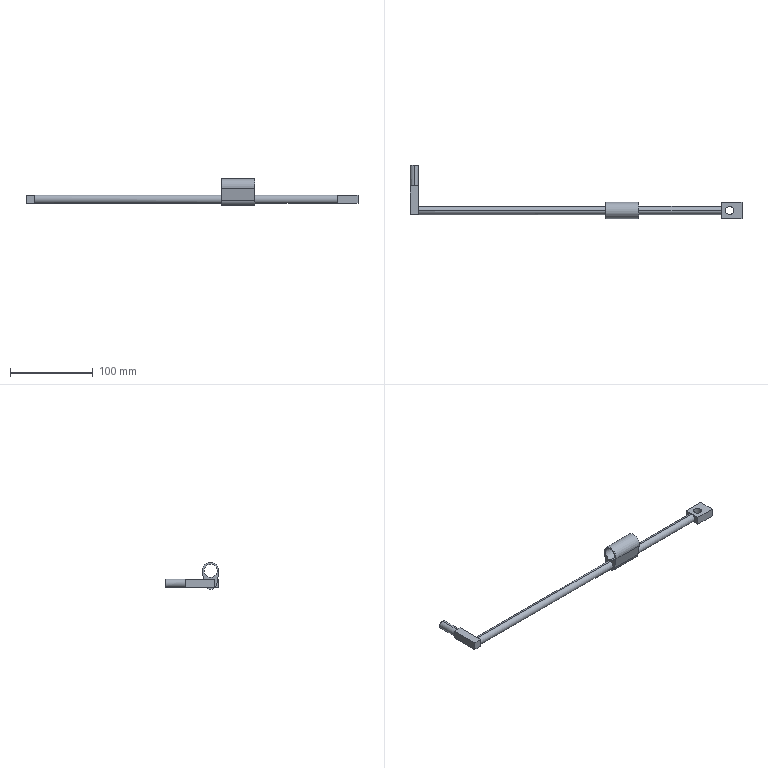Part | SolidWorks | features ICE 4, Extrusion 1, HoleWzd 1 | 1 solid | 40 faces | box 402 x 65 x 32.5 mm | volume 47736 mm3 | plane 23 | cylinder 15 | cone 2 | commonest cylinder face diameters 10 x8 3.3 x2 15 x2 16 x2 20 x1
STEP:
#1=CARTESIAN_POINT('',(-367.,10.,10.));
#2=VERTEX_POINT('',#1);
#3=CARTESIAN_POINT('',(-367.,10.,0.));
#4=VERTEX_POINT('',#3);
#5=CARTESIAN_POINT('',(-367.,10.,5.));
#6=DIRECTION('',(-1.,0.,0.));
#7=DIRECTION('',(0.,0.,1.));
#8=AXIS2_PLACEMENT_3D('',#5,#6,#7);
#9=CIRCLE('',#8,5.);
#10=EDGE_CURVE('',#2,#4,#9,.T.);
#11=ORIENTED_EDGE('',*,*,#10,.F.);
#12=CARTESIAN_POINT('',(-140.,10.,10.));
#13=VERTEX_POINT('',#12);
#14=CARTESIAN_POINT('',(-367.,10.,10.));
#15=DIRECTION('',(1.,0.,0.));
#16=VECTOR('',#15,1000.);
#17=LINE('',#14,#16);
#18=EDGE_CURVE('',#2,#13,#17,.T.);
#19=ORIENTED_EDGE('',*,*,#18,.T.);
#20=CARTESIAN_POINT('',(-140.,10.,0.));
#21=VERTEX_POINT('',#20);
#22=CARTESIAN_POINT('',(-140.,10.,5.));
#23=DIRECTION('',(-1.,0.,0.));
#24=DIRECTION('',(0.,0.,1.));
#25=AXIS2_PLACEMENT_3D('',#22,#23,#24);
#26=CIRCLE('',#25,5.);
#27=EDGE_CURVE('',#13,#21,#26,.T.);
#28=ORIENTED_EDGE('',*,*,#27,.T.);
#29=CARTESIAN_POINT('',(-367.,10.,0.));
#30=DIRECTION('',(1.,0.,0.));
#31=VECTOR('',#30,1000.);
#32=LINE('',#29,#31);
#33=EDGE_CURVE('',#4,#21,#32,.T.);
#34=ORIENTED_EDGE('',*,*,#33,.F.);
#35=EDGE_LOOP('',(#11,#19,#28,#34));
#36=FACE_OUTER_BOUND('',#35,.T.);
#37=CARTESIAN_POINT('',(-367.,10.,5.));
#38=DIRECTION('',(1.,0.,0.));
#39=DIRECTION('',(0.,0.,-1.));
#40=AXIS2_PLACEMENT_3D('',#37,#38,#39);
#41=CYLINDRICAL_SURFACE('',#40,5.);
#42=ADVANCED_FACE('',(#36),#41,.T.);
#43=CARTESIAN_POINT('',(-372.,65.,10.));
#44=VERTEX_POINT('',#43);
#45=CARTESIAN_POINT('',(-372.,65.,0.));
#46=VERTEX_POINT('',#45);
#47=CARTESIAN_POINT('',(-372.,65.,5.));
#48=DIRECTION('',(0.,1.,0.));
#49=DIRECTION('',(0.,0.,1.));
#50=AXIS2_PLACEMENT_3D('',#47,#48,#49);
#51=CIRCLE('',#50,5.);
#52=EDGE_CURVE('',#44,#46,#51,.T.);
#53=ORIENTED_EDGE('',*,*,#52,.F.);
#54=CARTESIAN_POINT('',(-372.,40.,10.));
#55=VERTEX_POINT('',#54);
#56=CARTESIAN_POINT('',(-372.,65.,10.));
#57=DIRECTION('',(0.,-1.,0.));
#58=VECTOR('',#57,1000.);
#59=LINE('',#56,#58);
#60=EDGE_CURVE('',#44,#55,#59,.T.);
#61=ORIENTED_EDGE('',*,*,#60,.T.);
#62=CARTESIAN_POINT('',(-367.,40.,5.));
#63=VERTEX_POINT('',#62);
#64=CARTESIAN_POINT('',(-372.,40.,5.));
#65=DIRECTION('',(0.,1.,0.));
#66=DIRECTION('',(0.,0.,1.));
#67=AXIS2_PLACEMENT_3D('',#64,#65,#66);
#68=CIRCLE('',#67,5.);
#69=EDGE_CURVE('',#55,#63,#68,.T.);
#70=ORIENTED_EDGE('',*,*,#69,.T.);
#71=CARTESIAN_POINT('',(-372.,40.,0.));
#72=VERTEX_POINT('',#71);
#73=CARTESIAN_POINT('',(-372.,40.,5.));
#74=DIRECTION('',(0.,1.,0.));
#75=DIRECTION('',(0.,0.,1.));
#76=AXIS2_PLACEMENT_3D('',#73,#74,#75);
#77=CIRCLE('',#76,5.);
#78=EDGE_CURVE('',#63,#72,#77,.T.);
#79=ORIENTED_EDGE('',*,*,#78,.T.);
#80=CARTESIAN_POINT('',(-372.,65.,0.));
#81=DIRECTION('',(0.,-1.,0.));
#82=VECTOR('',#81,1000.);
#83=LINE('',#80,#82);
#84=EDGE_CURVE('',#46,#72,#83,.T.);
#85=ORIENTED_EDGE('',*,*,#84,.F.);
#86=EDGE_LOOP('',(#53,#61,#70,#79,#85));
#87=FACE_OUTER_BOUND('',#86,.T.);
#88=CARTESIAN_POINT('',(-372.,65.,5.));
#89=DIRECTION('',(0.,-1.,0.));
#90=DIRECTION('',(0.,0.,-1.));
#91=AXIS2_PLACEMENT_3D('',#88,#89,#90);
#92=CYLINDRICAL_SURFACE('',#91,5.);
#93=ADVANCED_FACE('',(#87),#92,.T.);
#94=CARTESIAN_POINT('',(-140.,10.,12.));
#95=VERTEX_POINT('',#94);
#96=CARTESIAN_POINT('',(-140.,10.,28.));
#97=VERTEX_POINT('',#96);
#98=CARTESIAN_POINT('',(-140.,10.,20.));
#99=DIRECTION('',(-1.,0.,0.));
#100=DIRECTION('',(0.,0.,1.));
#101=AXIS2_PLACEMENT_3D('',#98,#99,#100);
#102=CIRCLE('',#101,8.);
#103=EDGE_CURVE('',#95,#97,#102,.T.);
#104=ORIENTED_EDGE('',*,*,#103,.T.);
#105=CARTESIAN_POINT('',(-100.,10.,28.));
#106=VERTEX_POINT('',#105);
#107=CARTESIAN_POINT('',(-140.,10.,28.));
#108=DIRECTION('',(1.,0.,0.));
#109=VECTOR('',#108,1000.);
#110=LINE('',#107,#109);
#111=EDGE_CURVE('',#97,#106,#110,.T.);
#112=ORIENTED_EDGE('',*,*,#111,.T.);
#113=CARTESIAN_POINT('',(-100.,10.,12.));
#114=VERTEX_POINT('',#113);
#115=CARTESIAN_POINT('',(-100.,10.,20.));
#116=DIRECTION('',(-1.,0.,0.));
#117=DIRECTION('',(0.,0.,1.));
#118=AXIS2_PLACEMENT_3D('',#115,#116,#117);
#119=CIRCLE('',#118,8.);
#120=EDGE_CURVE('',#114,#106,#119,.T.);
#121=ORIENTED_EDGE('',*,*,#120,.F.);
#122=CARTESIAN_POINT('',(-140.,10.,12.));
#123=DIRECTION('',(1.,0.,0.));
#124=VECTOR('',#123,1000.);
#125=LINE('',#122,#124);
#126=EDGE_CURVE('',#95,#114,#125,.T.);
#127=ORIENTED_EDGE('',*,*,#126,.F.);
#128=EDGE_LOOP('',(#104,#112,#121,#127));
#129=FACE_OUTER_BOUND('',#128,.T.);
#130=CARTESIAN_POINT('',(-140.,10.,20.));
#131=DIRECTION('',(1.,0.,0.));
#132=DIRECTION('',(0.,0.,-1.));
#133=AXIS2_PLACEMENT_3D('',#130,#131,#132);
#134=CYLINDRICAL_SURFACE('',#133,8.);
#135=ADVANCED_FACE('',(#129),#134,.F.);
#136=CARTESIAN_POINT('',(-140.,10.,-2.5));
#137=VERTEX_POINT('',#136);
#138=CARTESIAN_POINT('',(-140.,2.605,3.75));
#139=VERTEX_POINT('',#138);
#140=CARTESIAN_POINT('',(-140.,10.,5.));
#141=DIRECTION('',(-1.,0.,0.));
#142=DIRECTION('',(0.,0.,1.));
#143=AXIS2_PLACEMENT_3D('',#140,#141,#142);
#144=CIRCLE('',#143,7.5);
#145=EDGE_CURVE('',#137,#139,#144,.T.);
#146=ORIENTED_EDGE('',*,*,#145,.F.);
#147=CARTESIAN_POINT('',(-100.,10.,-2.5));
#148=VERTEX_POINT('',#147);
#149=CARTESIAN_POINT('',(-140.,10.,-2.5));
#150=DIRECTION('',(1.,0.,0.));
#151=VECTOR('',#150,1000.);
#152=LINE('',#149,#151);
#153=EDGE_CURVE('',#137,#148,#152,.T.);
#154=ORIENTED_EDGE('',*,*,#153,.T.);
#155=CARTESIAN_POINT('',(-100.,2.605,3.75));
#156=VERTEX_POINT('',#155);
#157=CARTESIAN_POINT('',(-100.,10.,5.));
#158=DIRECTION('',(-1.,0.,0.));
#159=DIRECTION('',(0.,0.,1.));
#160=AXIS2_PLACEMENT_3D('',#157,#158,#159);
#161=CIRCLE('',#160,7.5);
#162=EDGE_CURVE('',#148,#156,#161,.T.);
#163=ORIENTED_EDGE('',*,*,#162,.T.);
#164=CARTESIAN_POINT('',(-140.,2.605,3.75));
#165=DIRECTION('',(1.,0.,0.));
#166=VECTOR('',#165,1000.);
#167=LINE('',#164,#166);
#168=EDGE_CURVE('',#139,#156,#167,.T.);
#169=ORIENTED_EDGE('',*,*,#168,.F.);
#170=EDGE_LOOP('',(#146,#154,#163,#169));
#171=FACE_OUTER_BOUND('',#170,.T.);
#172=CARTESIAN_POINT('',(-140.,10.,5.));
#173=DIRECTION('',(1.,0.,0.));
#174=DIRECTION('',(0.,0.,-1.));
#175=AXIS2_PLACEMENT_3D('',#172,#173,#174);
#176=CYLINDRICAL_SURFACE('',#175,7.5);
#177=ADVANCED_FACE('',(#171),#176,.T.);
#178=CARTESIAN_POINT('',(20.,10.,6.65));
#179=VERTEX_POINT('',#178);
#180=CARTESIAN_POINT('',(20.,10.,3.35));
#181=VERTEX_POINT('',#180);
#182=CARTESIAN_POINT('',(20.,10.,5.));
#183=DIRECTION('',(1.,0.,0.));
#184=DIRECTION('',(0.,0.,-1.));
#185=AXIS2_PLACEMENT_3D('',#182,#183,#184);
#186=CIRCLE('',#185,1.65);
#187=EDGE_CURVE('',#179,#181,#186,.T.);
#188=ORIENTED_EDGE('',*,*,#187,.F.);
#189=CARTESIAN_POINT('',(25.,10.,6.65));
#190=VERTEX_POINT('',#189);
#191=CARTESIAN_POINT('',(25.,10.,6.65));
#192=DIRECTION('',(1.,0.,0.));
#193=VECTOR('',#192,1000.);
#194=LINE('',#191,#193);
#195=EDGE_CURVE('',#179,#190,#194,.T.);
#196=ORIENTED_EDGE('',*,*,#195,.T.);
#197=CARTESIAN_POINT('',(25.,10.,3.35));
#198=VERTEX_POINT('',#197);
#199=CARTESIAN_POINT('',(25.,10.,5.));
#200=DIRECTION('',(1.,0.,0.));
#201=DIRECTION('',(0.,0.,-1.));
#202=AXIS2_PLACEMENT_3D('',#199,#200,#201);
#203=CIRCLE('',#202,1.65);
#204=EDGE_CURVE('',#190,#198,#203,.T.);
#205=ORIENTED_EDGE('',*,*,#204,.T.);
#206=CARTESIAN_POINT('',(25.,10.,3.35));
#207=DIRECTION('',(1.,0.,0.));
#208=VECTOR('',#207,1000.);
#209=LINE('',#206,#208);
#210=EDGE_CURVE('',#181,#198,#209,.T.);
#211=ORIENTED_EDGE('',*,*,#210,.F.);
#212=EDGE_LOOP('',(#188,#196,#205,#211));
#213=FACE_OUTER_BOUND('',#212,.T.);
#214=CARTESIAN_POINT('',(25.,10.,5.));
#215=DIRECTION('',(1.,0.,0.));
#216=DIRECTION('',(0.,0.,-1.));
#217=AXIS2_PLACEMENT_3D('',#214,#215,#216);
#218=CYLINDRICAL_SURFACE('',#217,1.65);
#219=ADVANCED_FACE('',(#213),#218,.F.);
#220=CARTESIAN_POINT('',(19.009,10.,5.));
#221=VERTEX_POINT('',#220);
#222=CARTESIAN_POINT('',(20.,10.,3.35));
#223=DIRECTION('',(0.515,0.,-0.8572));
#224=VECTOR('',#223,1000.);
#225=LINE('',#222,#224);
#226=EDGE_CURVE('',#221,#181,#225,.T.);
#227=ORIENTED_EDGE('',*,*,#226,.F.);
#228=CARTESIAN_POINT('',(20.,10.,6.65));
#229=DIRECTION('',(0.515,0.,0.8572));
#230=VECTOR('',#229,1000.);
#231=LINE('',#228,#230);
#232=EDGE_CURVE('',#221,#179,#231,.T.);
#233=ORIENTED_EDGE('',*,*,#232,.T.);
#234=ORIENTED_EDGE('',*,*,#187,.T.);
#235=EDGE_LOOP('',(#227,#233,#234));
#236=FACE_OUTER_BOUND('',#235,.T.);
#237=CARTESIAN_POINT('',(20.,10.,5.));
#238=DIRECTION('',(1.,0.,0.));
#239=DIRECTION('',(0.,0.,-1.));
#240=AXIS2_PLACEMENT_3D('',#237,#238,#239);
#241=CONICAL_SURFACE('',#240,1.65,1.03);
#242=ADVANCED_FACE('',(#236),#241,.F.);
#243=CARTESIAN_POINT('',(5.,10.,10.));
#244=VERTEX_POINT('',#243);
#245=CARTESIAN_POINT('',(15.,10.,10.));
#246=VERTEX_POINT('',#245);
#247=CARTESIAN_POINT('',(10.,10.,10.));
#248=DIRECTION('',(0.,0.,1.));
#249=DIRECTION('',(1.,0.,0.));
#250=AXIS2_PLACEMENT_3D('',#247,#248,#249);
#251=CIRCLE('',#250,5.);
#252=EDGE_CURVE('',#244,#246,#251,.T.);
#253=ORIENTED_EDGE('',*,*,#252,.T.);
#254=CARTESIAN_POINT('',(15.,10.,0.));
#255=VERTEX_POINT('',#254);
#256=CARTESIAN_POINT('',(15.,10.,10.));
#257=DIRECTION('',(0.,0.,-1.));
#258=VECTOR('',#257,1000.);
#259=LINE('',#256,#258);
#260=EDGE_CURVE('',#246,#255,#259,.T.);
#261=ORIENTED_EDGE('',*,*,#260,.T.);
#262=CARTESIAN_POINT('',(5.,10.,0.));
#263=VERTEX_POINT('',#262);
#264=CARTESIAN_POINT('',(10.,10.,0.));
#265=DIRECTION('',(0.,0.,1.));
#266=DIRECTION('',(1.,0.,0.));
#267=AXIS2_PLACEMENT_3D('',#264,#265,#266);
#268=CIRCLE('',#267,5.);
#269=EDGE_CURVE('',#263,#255,#268,.T.);
#270=ORIENTED_EDGE('',*,*,#269,.F.);
#271=CARTESIAN_POINT('',(5.,10.,10.));
#272=DIRECTION('',(0.,0.,-1.));
#273=VECTOR('',#272,1000.);
#274=LINE('',#271,#273);
#275=EDGE_CURVE('',#244,#263,#274,.T.);
#276=ORIENTED_EDGE('',*,*,#275,.F.);
#277=EDGE_LOOP('',(#253,#261,#270,#276));
#278=FACE_OUTER_BOUND('',#277,.T.);
#279=CARTESIAN_POINT('',(10.,10.,10.));
#280=DIRECTION('',(0.,0.,-1.));
#281=DIRECTION('',(-1.,0.,0.));
#282=AXIS2_PLACEMENT_3D('',#279,#280,#281);
#283=CYLINDRICAL_SURFACE('',#282,5.);
#284=ADVANCED_FACE('',(#278),#283,.F.);
#285=CARTESIAN_POINT('',(-100.,10.,10.));
#286=VERTEX_POINT('',#285);
#287=CARTESIAN_POINT('',(-100.,10.,0.));
#288=VERTEX_POINT('',#287);
#289=CARTESIAN_POINT('',(-100.,10.,5.));
#290=DIRECTION('',(-1.,0.,0.));
#291=DIRECTION('',(0.,0.,1.));
#292=AXIS2_PLACEMENT_3D('',#289,#290,#291);
#293=CIRCLE('',#292,5.);
#294=EDGE_CURVE('',#286,#288,#293,.T.);
#295=ORIENTED_EDGE('',*,*,#294,.F.);
#296=CARTESIAN_POINT('',(0.,10.,10.));
#297=VERTEX_POINT('',#296);
#298=CARTESIAN_POINT('',(-367.,10.,10.));
#299=DIRECTION('',(1.,0.,0.));
#300=VECTOR('',#299,1000.);
#301=LINE('',#298,#300);
#302=EDGE_CURVE('',#286,#297,#301,.T.);
#303=ORIENTED_EDGE('',*,*,#302,.T.);
#304=CARTESIAN_POINT('',(0.,10.,0.));
#305=VERTEX_POINT('',#304);
#306=CARTESIAN_POINT('',(0.,10.,5.));
#307=DIRECTION('',(-1.,0.,0.));
#308=DIRECTION('',(0.,0.,1.));
#309=AXIS2_PLACEMENT_3D('',#306,#307,#308);
#310=CIRCLE('',#309,5.);
#311=EDGE_CURVE('',#297,#305,#310,.T.);
#312=ORIENTED_EDGE('',*,*,#311,.T.);
#313=CARTESIAN_POINT('',(-367.,10.,0.));
#314=DIRECTION('',(1.,0.,0.));
#315=VECTOR('',#314,1000.);
#316=LINE('',#313,#315);
#317=EDGE_CURVE('',#288,#305,#316,.T.);
#318=ORIENTED_EDGE('',*,*,#317,.F.);
#319=EDGE_LOOP('',(#295,#303,#312,#318));
#320=FACE_OUTER_BOUND('',#319,.T.);
#321=CARTESIAN_POINT('',(-367.,10.,5.));
#322=DIRECTION('',(1.,0.,0.));
#323=DIRECTION('',(0.,0.,-1.));
#324=AXIS2_PLACEMENT_3D('',#321,#322,#323);
#325=CYLINDRICAL_SURFACE('',#324,5.);
#326=ADVANCED_FACE('',(#320),#325,.T.);
#327=ORIENTED_EDGE('',*,*,#302,.F.);
#328=CARTESIAN_POINT('',(-100.,10.,5.));
#329=DIRECTION('',(-1.,0.,0.));
#330=DIRECTION('',(0.,0.,1.));
#331=AXIS2_PLACEMENT_3D('',#328,#329,#330);
#332=CIRCLE('',#331,5.);
#333=EDGE_CURVE('',#288,#286,#332,.T.);
#334=ORIENTED_EDGE('',*,*,#333,.F.);
#335=ORIENTED_EDGE('',*,*,#317,.T.);
#336=CARTESIAN_POINT('',(0.,10.,5.));
#337=DIRECTION('',(-1.,0.,0.));
#338=DIRECTION('',(0.,0.,1.));
#339=AXIS2_PLACEMENT_3D('',#336,#337,#338);
#340=CIRCLE('',#339,5.);
#341=EDGE_CURVE('',#305,#297,#340,.T.);
#342=ORIENTED_EDGE('',*,*,#341,.T.);
#343=EDGE_LOOP('',(#327,#334,#335,#342));
#344=FACE_OUTER_BOUND('',#343,.T.);
#345=CARTESIAN_POINT('',(-367.,10.,5.));
#346=DIRECTION('',(1.,0.,0.));
#347=DIRECTION('',(0.,0.,-1.));
#348=AXIS2_PLACEMENT_3D('',#345,#346,#347);
#349=CYLINDRICAL_SURFACE('',#348,5.);
#350=ADVANCED_FACE('',(#344),#349,.T.);
#351=ORIENTED_EDGE('',*,*,#311,.F.);
#352=CARTESIAN_POINT('',(0.,20.,10.));
#353=VERTEX_POINT('',#352);
#354=CARTESIAN_POINT('',(0.,0.,10.));
#355=DIRECTION('',(0.,-1.,0.));
#356=VECTOR('',#355,1000.);
#357=LINE('',#354,#356);
#358=EDGE_CURVE('',#353,#297,#357,.T.);
#359=ORIENTED_EDGE('',*,*,#358,.F.);
#360=CARTESIAN_POINT('',(0.,20.,0.));
#361=VERTEX_POINT('',#360);
#362=CARTESIAN_POINT('',(0.,20.,10.));
#363=DIRECTION('',(0.,0.,-1.));
#364=VECTOR('',#363,1000.);
#365=LINE('',#362,#364);
#366=EDGE_CURVE('',#353,#361,#365,.T.);
#367=ORIENTED_EDGE('',*,*,#366,.T.);
#368=CARTESIAN_POINT('',(0.,0.,0.));
#369=DIRECTION('',(0.,-1.,0.));
#370=VECTOR('',#369,1000.);
#371=LINE('',#368,#370);
#372=EDGE_CURVE('',#361,#305,#371,.T.);
#373=ORIENTED_EDGE('',*,*,#372,.T.);
#374=EDGE_LOOP('',(#351,#359,#367,#373));
#375=FACE_OUTER_BOUND('',#374,.T.);
#376=CARTESIAN_POINT('',(0.,0.,10.));
#377=DIRECTION('',(1.,0.,0.));
#378=DIRECTION('',(0.,0.,-1.));
#379=AXIS2_PLACEMENT_3D('',#376,#377,#378);
#380=PLANE('',#379);
#381=ADVANCED_FACE('',(#375),#380,.F.);
#382=ORIENTED_EDGE('',*,*,#341,.F.);
#383=CARTESIAN_POINT('',(0.,0.,0.));
#384=VERTEX_POINT('',#383);
#385=CARTESIAN_POINT('',(0.,0.,0.));
#386=DIRECTION('',(0.,-1.,0.));
#387=VECTOR('',#386,1000.);
#388=LINE('',#385,#387);
#389=EDGE_CURVE('',#305,#384,#388,.T.);
#390=ORIENTED_EDGE('',*,*,#389,.T.);
#391=CARTESIAN_POINT('',(0.,0.,10.));
#392=VERTEX_POINT('',#391);
#393=CARTESIAN_POINT('',(0.,0.,10.));
#394=DIRECTION('',(0.,0.,-1.));
#395=VECTOR('',#394,1000.);
#396=LINE('',#393,#395);
#397=EDGE_CURVE('',#392,#384,#396,.T.);
#398=ORIENTED_EDGE('',*,*,#397,.F.);
#399=CARTESIAN_POINT('',(0.,0.,10.));
#400=DIRECTION('',(0.,-1.,0.));
#401=VECTOR('',#400,1000.);
#402=LINE('',#399,#401);
#403=EDGE_CURVE('',#297,#392,#402,.T.);
#404=ORIENTED_EDGE('',*,*,#403,.F.);
#405=EDGE_LOOP('',(#382,#390,#398,#404));
#406=FACE_OUTER_BOUND('',#405,.T.);
#407=CARTESIAN_POINT('',(0.,0.,10.));
#408=DIRECTION('',(1.,0.,0.));
#409=DIRECTION('',(0.,0.,-1.));
#410=AXIS2_PLACEMENT_3D('',#407,#408,#409);
#411=PLANE('',#410);
#412=ADVANCED_FACE('',(#406),#411,.F.);
#413=ORIENTED_EDGE('',*,*,#358,.T.);
#414=ORIENTED_EDGE('',*,*,#403,.T.);
#415=CARTESIAN_POINT('',(25.,0.,10.));
#416=VERTEX_POINT('',#415);
#417=CARTESIAN_POINT('',(0.,0.,10.));
#418=DIRECTION('',(1.,0.,0.));
#419=VECTOR('',#418,1000.);
#420=LINE('',#417,#419);
#421=EDGE_CURVE('',#392,#416,#420,.T.);
#422=ORIENTED_EDGE('',*,*,#421,.T.);
#423=CARTESIAN_POINT('',(25.,20.,10.));
#424=VERTEX_POINT('',#423);
#425=CARTESIAN_POINT('',(25.,0.,10.));
#426=DIRECTION('',(0.,1.,0.));
#427=VECTOR('',#426,1000.);
#428=LINE('',#425,#427);
#429=EDGE_CURVE('',#416,#424,#428,.T.);
#430=ORIENTED_EDGE('',*,*,#429,.T.);
#431=CARTESIAN_POINT('',(0.,20.,10.));
#432=DIRECTION('',(-1.,0.,0.));
#433=VECTOR('',#432,1000.);
#434=LINE('',#431,#433);
#435=EDGE_CURVE('',#424,#353,#434,.T.);
#436=ORIENTED_EDGE('',*,*,#435,.T.);
#437=EDGE_LOOP('',(#413,#414,#422,#430,#436));
#438=FACE_OUTER_BOUND('',#437,.T.);
#439=ORIENTED_EDGE('',*,*,#252,.F.);
#440=CARTESIAN_POINT('',(10.,10.,10.));
#441=DIRECTION('',(0.,0.,1.));
#442=DIRECTION('',(1.,0.,0.));
#443=AXIS2_PLACEMENT_3D('',#440,#441,#442);
#444=CIRCLE('',#443,5.);
#445=EDGE_CURVE('',#246,#244,#444,.T.);
#446=ORIENTED_EDGE('',*,*,#445,.F.);
#447=EDGE_LOOP('',(#439,#446));
#448=FACE_BOUND('',#447,.T.);
#449=CARTESIAN_POINT('',(0.,0.,10.));
#450=DIRECTION('',(0.,0.,-1.));
#451=DIRECTION('',(-1.,0.,0.));
#452=AXIS2_PLACEMENT_3D('',#449,#450,#451);
#453=PLANE('',#452);
#454=ADVANCED_FACE('',(#438,#448),#453,.F.);
#455=ORIENTED_EDGE('',*,*,#372,.F.);
#456=CARTESIAN_POINT('',(25.,20.,0.));
#457=VERTEX_POINT('',#456);
#458=CARTESIAN_POINT('',(0.,20.,0.));
#459=DIRECTION('',(-1.,0.,0.));
#460=VECTOR('',#459,1000.);
#461=LINE('',#458,#460);
#462=EDGE_CURVE('',#457,#361,#461,.T.);
#463=ORIENTED_EDGE('',*,*,#462,.F.);
#464=CARTESIAN_POINT('',(25.,0.,0.));
#465=VERTEX_POINT('',#464);
#466=CARTESIAN_POINT('',(25.,0.,0.));
#467=DIRECTION('',(0.,1.,0.));
#468=VECTOR('',#467,1000.);
#469=LINE('',#466,#468);
#470=EDGE_CURVE('',#465,#457,#469,.T.);
#471=ORIENTED_EDGE('',*,*,#470,.F.);
#472=CARTESIAN_POINT('',(0.,0.,0.));
#473=DIRECTION('',(1.,0.,0.));
#474=VECTOR('',#473,1000.);
#475=LINE('',#472,#474);
#476=EDGE_CURVE('',#384,#465,#475,.T.);
#477=ORIENTED_EDGE('',*,*,#476,.F.);
#478=ORIENTED_EDGE('',*,*,#389,.F.);
#479=EDGE_LOOP('',(#455,#463,#471,#477,#478));
#480=FACE_OUTER_BOUND('',#479,.T.);
#481=ORIENTED_EDGE('',*,*,#269,.T.);
#482=CARTESIAN_POINT('',(10.,10.,0.));
#483=DIRECTION('',(0.,0.,1.));
#484=DIRECTION('',(1.,0.,0.));
#485=AXIS2_PLACEMENT_3D('',#482,#483,#484);
#486=CIRCLE('',#485,5.);
#487=EDGE_CURVE('',#255,#263,#486,.T.);
#488=ORIENTED_EDGE('',*,*,#487,.T.);
#489=EDGE_LOOP('',(#481,#488));
#490=FACE_BOUND('',#489,.T.);
#491=CARTESIAN_POINT('',(0.,0.,0.));
#492=DIRECTION('',(0.,0.,-1.));
#493=DIRECTION('',(-1.,0.,0.));
#494=AXIS2_PLACEMENT_3D('',#491,#492,#493);
#495=PLANE('',#494);
#496=ADVANCED_FACE('',(#480,#490),#495,.T.);
#497=ORIENTED_EDGE('',*,*,#476,.T.);
#498=CARTESIAN_POINT('',(25.,0.,10.));
#499=DIRECTION('',(0.,0.,-1.));
#500=VECTOR('',#499,1000.);
#501=LINE('',#498,#500);
#502=EDGE_CURVE('',#416,#465,#501,.T.);
#503=ORIENTED_EDGE('',*,*,#502,.F.);
#504=ORIENTED_EDGE('',*,*,#421,.F.);
#505=ORIENTED_EDGE('',*,*,#397,.T.);
#506=EDGE_LOOP('',(#497,#503,#504,#505));
#507=FACE_OUTER_BOUND('',#506,.T.);
#508=CARTESIAN_POINT('',(0.,0.,10.));
#509=DIRECTION('',(0.,1.,0.));
#510=DIRECTION('',(0.,0.,1.));
#511=AXIS2_PLACEMENT_3D('',#508,#509,#510);
#512=PLANE('',#511);
#513=ADVANCED_FACE('',(#507),#512,.F.);
#514=CARTESIAN_POINT('',(25.,10.,5.));
#515=DIRECTION('',(1.,0.,0.));
#516=DIRECTION('',(0.,0.,-1.));
#517=AXIS2_PLACEMENT_3D('',#514,#515,#516);
#518=CIRCLE('',#517,1.65);
#519=EDGE_CURVE('',#198,#190,#518,.T.);
#520=ORIENTED_EDGE('',*,*,#519,.F.);
#521=ORIENTED_EDGE('',*,*,#204,.F.);
#522=EDGE_LOOP('',(#520,#521));
#523=FACE_BOUND('',#522,.T.);
#524=ORIENTED_EDGE('',*,*,#470,.T.);
#525=CARTESIAN_POINT('',(25.,20.,10.));
#526=DIRECTION('',(0.,0.,-1.));
#527=VECTOR('',#526,1000.);
#528=LINE('',#525,#527);
#529=EDGE_CURVE('',#424,#457,#528,.T.);
#530=ORIENTED_EDGE('',*,*,#529,.F.);
#531=ORIENTED_EDGE('',*,*,#429,.F.);
#532=ORIENTED_EDGE('',*,*,#502,.T.);
#533=EDGE_LOOP('',(#524,#530,#531,#532));
#534=FACE_OUTER_BOUND('',#533,.T.);
#535=CARTESIAN_POINT('',(25.,0.,10.));
#536=DIRECTION('',(-1.,0.,0.));
#537=DIRECTION('',(0.,0.,1.));
#538=AXIS2_PLACEMENT_3D('',#535,#536,#537);
#539=PLANE('',#538);
#540=ADVANCED_FACE('',(#523,#534),#539,.F.);
#541=ORIENTED_EDGE('',*,*,#462,.T.);
#542=ORIENTED_EDGE('',*,*,#366,.F.);
#543=ORIENTED_EDGE('',*,*,#435,.F.);
#544=ORIENTED_EDGE('',*,*,#529,.T.);
#545=EDGE_LOOP('',(#541,#542,#543,#544));
#546=FACE_OUTER_BOUND('',#545,.T.);
#547=CARTESIAN_POINT('',(0.,20.,10.));
#548=DIRECTION('',(0.,-1.,0.));
#549=DIRECTION('',(0.,0.,-1.));
#550=AXIS2_PLACEMENT_3D('',#547,#548,#549);
#551=PLANE('',#550);
#552=ADVANCED_FACE('',(#546),#551,.F.);
#553=ORIENTED_EDGE('',*,*,#260,.F.);
#554=ORIENTED_EDGE('',*,*,#445,.T.);
#555=ORIENTED_EDGE('',*,*,#275,.T.);
#556=ORIENTED_EDGE('',*,*,#487,.F.);
#557=EDGE_LOOP('',(#553,#554,#555,#556));
#558=FACE_OUTER_BOUND('',#557,.T.);
#559=CARTESIAN_POINT('',(10.,10.,10.));
#560=DIRECTION('',(0.,0.,-1.));
#561=DIRECTION('',(-1.,0.,0.));
#562=AXIS2_PLACEMENT_3D('',#559,#560,#561);
#563=CYLINDRICAL_SURFACE('',#562,5.);
#564=ADVANCED_FACE('',(#558),#563,.F.);
#565=ORIENTED_EDGE('',*,*,#232,.F.);
#566=ORIENTED_EDGE('',*,*,#226,.T.);
#567=CARTESIAN_POINT('',(20.,10.,5.));
#568=DIRECTION('',(1.,0.,0.));
#569=DIRECTION('',(0.,0.,-1.));
#570=AXIS2_PLACEMENT_3D('',#567,#568,#569);
#571=CIRCLE('',#570,1.65);
#572=EDGE_CURVE('',#181,#179,#571,.T.);
#573=ORIENTED_EDGE('',*,*,#572,.T.);
#574=EDGE_LOOP('',(#565,#566,#573));
#575=FACE_OUTER_BOUND('',#574,.T.);
#576=CARTESIAN_POINT('',(20.,10.,5.));
#577=DIRECTION('',(1.,0.,0.));
#578=DIRECTION('',(0.,0.,-1.));
#579=AXIS2_PLACEMENT_3D('',#576,#577,#578);
#580=CONICAL_SURFACE('',#579,1.65,1.03);
#581=ADVANCED_FACE('',(#575),#580,.F.);
#582=ORIENTED_EDGE('',*,*,#195,.F.);
#583=ORIENTED_EDGE('',*,*,#572,.F.);
#584=ORIENTED_EDGE('',*,*,#210,.T.);
#585=ORIENTED_EDGE('',*,*,#519,.T.);
#586=EDGE_LOOP('',(#582,#583,#584,#585));
#587=FACE_OUTER_BOUND('',#586,.T.);
#588=CARTESIAN_POINT('',(25.,10.,5.));
#589=DIRECTION('',(1.,0.,0.));
#590=DIRECTION('',(0.,0.,-1.));
#591=AXIS2_PLACEMENT_3D('',#588,#589,#590);
#592=CYLINDRICAL_SURFACE('',#591,1.65);
#593=ADVANCED_FACE('',(#587),#592,.F.);
#594=ORIENTED_EDGE('',*,*,#103,.F.);
#595=CARTESIAN_POINT('',(-140.,10.,20.));
#596=DIRECTION('',(-1.,0.,0.));
#597=DIRECTION('',(0.,0.,1.));
#598=AXIS2_PLACEMENT_3D('',#595,#596,#597);
#599=CIRCLE('',#598,8.);
#600=EDGE_CURVE('',#97,#95,#599,.T.);
#601=ORIENTED_EDGE('',*,*,#600,.F.);
#602=EDGE_LOOP('',(#594,#601));
#603=FACE_BOUND('',#602,.T.);
#604=CARTESIAN_POINT('',(-140.,17.395,3.75));
#605=VERTEX_POINT('',#604);
#606=CARTESIAN_POINT('',(-140.,10.,5.));
#607=DIRECTION('',(-1.,0.,0.));
#608=DIRECTION('',(0.,0.,1.));
#609=AXIS2_PLACEMENT_3D('',#606,#607,#608);
#610=CIRCLE('',#609,7.5);
#611=EDGE_CURVE('',#605,#137,#610,.T.);
#612=ORIENTED_EDGE('',*,*,#611,.T.);
#613=ORIENTED_EDGE('',*,*,#145,.T.);
#614=CARTESIAN_POINT('',(-140.,0.1399,18.333));
#615=VERTEX_POINT('',#614);
#616=CARTESIAN_POINT('',(-140.,2.605,3.75));
#617=DIRECTION('',(0.,-0.1667,0.986));
#618=VECTOR('',#617,1000.);
#619=LINE('',#616,#618);
#620=EDGE_CURVE('',#139,#615,#619,.T.);
#621=ORIENTED_EDGE('',*,*,#620,.T.);
#622=CARTESIAN_POINT('',(-140.,19.86,18.333));
#623=VERTEX_POINT('',#622);
#624=CARTESIAN_POINT('',(-140.,10.,20.));
#625=DIRECTION('',(-1.,0.,0.));
#626=DIRECTION('',(0.,0.,1.));
#627=AXIS2_PLACEMENT_3D('',#624,#625,#626);
#628=CIRCLE('',#627,10.);
#629=EDGE_CURVE('',#615,#623,#628,.T.);
#630=ORIENTED_EDGE('',*,*,#629,.T.);
#631=CARTESIAN_POINT('',(-140.,17.395,3.75));
#632=DIRECTION('',(0.,-0.1667,-0.986));
#633=VECTOR('',#632,1000.);
#634=LINE('',#631,#633);
#635=EDGE_CURVE('',#623,#605,#634,.T.);
#636=ORIENTED_EDGE('',*,*,#635,.T.);
#637=EDGE_LOOP('',(#612,#613,#621,#630,#636));
#638=FACE_OUTER_BOUND('',#637,.T.);
#639=CARTESIAN_POINT('',(-140.,10.,5.));
#640=DIRECTION('',(-1.,0.,0.));
#641=DIRECTION('',(0.,0.,1.));
#642=AXIS2_PLACEMENT_3D('',#639,#640,#641);
#643=CIRCLE('',#642,5.);
#644=EDGE_CURVE('',#21,#13,#643,.T.);
#645=ORIENTED_EDGE('',*,*,#644,.F.);
#646=ORIENTED_EDGE('',*,*,#27,.F.);
#647=EDGE_LOOP('',(#645,#646));
#648=FACE_BOUND('',#647,.T.);
#649=CARTESIAN_POINT('',(-140.,10.,5.));
#650=DIRECTION('',(-1.,0.,0.));
#651=DIRECTION('',(0.,0.,1.));
#652=AXIS2_PLACEMENT_3D('',#649,#650,#651);
#653=PLANE('',#652);
#654=ADVANCED_FACE('',(#603,#638,#648),#653,.T.);
#655=ORIENTED_EDGE('',*,*,#120,.T.);
#656=CARTESIAN_POINT('',(-100.,10.,20.));
#657=DIRECTION('',(-1.,0.,0.));
#658=DIRECTION('',(0.,0.,1.));
#659=AXIS2_PLACEMENT_3D('',#656,#657,#658);
#660=CIRCLE('',#659,8.);
#661=EDGE_CURVE('',#106,#114,#660,.T.);
#662=ORIENTED_EDGE('',*,*,#661,.T.);
#663=EDGE_LOOP('',(#655,#662));
#664=FACE_BOUND('',#663,.T.);
#665=CARTESIAN_POINT('',(-100.,17.395,3.75));
#666=VERTEX_POINT('',#665);
#667=CARTESIAN_POINT('',(-100.,10.,5.));
#668=DIRECTION('',(-1.,0.,0.));
#669=DIRECTION('',(0.,0.,1.));
#670=AXIS2_PLACEMENT_3D('',#667,#668,#669);
#671=CIRCLE('',#670,7.5);
#672=EDGE_CURVE('',#666,#148,#671,.T.);
#673=ORIENTED_EDGE('',*,*,#672,.F.);
#674=CARTESIAN_POINT('',(-100.,19.86,18.333));
#675=VERTEX_POINT('',#674);
#676=CARTESIAN_POINT('',(-100.,17.395,3.75));
#677=DIRECTION('',(0.,-0.1667,-0.986));
#678=VECTOR('',#677,1000.);
#679=LINE('',#676,#678);
#680=EDGE_CURVE('',#675,#666,#679,.T.);
#681=ORIENTED_EDGE('',*,*,#680,.F.);
#682=CARTESIAN_POINT('',(-100.,0.1399,18.333));
#683=VERTEX_POINT('',#682);
#684=CARTESIAN_POINT('',(-100.,10.,20.));
#685=DIRECTION('',(-1.,0.,0.));
#686=DIRECTION('',(0.,0.,1.));
#687=AXIS2_PLACEMENT_3D('',#684,#685,#686);
#688=CIRCLE('',#687,10.);
#689=EDGE_CURVE('',#683,#675,#688,.T.);
#690=ORIENTED_EDGE('',*,*,#689,.F.);
#691=CARTESIAN_POINT('',(-100.,2.605,3.75));
#692=DIRECTION('',(0.,-0.1667,0.986));
#693=VECTOR('',#692,1000.);
#694=LINE('',#691,#693);
#695=EDGE_CURVE('',#156,#683,#694,.T.);
#696=ORIENTED_EDGE('',*,*,#695,.F.);
#697=ORIENTED_EDGE('',*,*,#162,.F.);
#698=EDGE_LOOP('',(#673,#681,#690,#696,#697));
#699=FACE_OUTER_BOUND('',#698,.T.);
#700=ORIENTED_EDGE('',*,*,#333,.T.);
#701=ORIENTED_EDGE('',*,*,#294,.T.);
#702=EDGE_LOOP('',(#700,#701));
#703=FACE_BOUND('',#702,.T.);
#704=CARTESIAN_POINT('',(-100.,10.,5.));
#705=DIRECTION('',(-1.,0.,0.));
#706=DIRECTION('',(0.,0.,1.));
#707=AXIS2_PLACEMENT_3D('',#704,#705,#706);
#708=PLANE('',#707);
#709=ADVANCED_FACE('',(#664,#699,#703),#708,.F.);
#710=ORIENTED_EDGE('',*,*,#153,.F.);
#711=ORIENTED_EDGE('',*,*,#611,.F.);
#712=CARTESIAN_POINT('',(-140.,17.395,3.75));
#713=DIRECTION('',(1.,0.,0.));
#714=VECTOR('',#713,1000.);
#715=LINE('',#712,#714);
#716=EDGE_CURVE('',#605,#666,#715,.T.);
#717=ORIENTED_EDGE('',*,*,#716,.T.);
#718=ORIENTED_EDGE('',*,*,#672,.T.);
#719=EDGE_LOOP('',(#710,#711,#717,#718));
#720=FACE_OUTER_BOUND('',#719,.T.);
#721=CARTESIAN_POINT('',(-140.,10.,5.));
#722=DIRECTION('',(1.,0.,0.));
#723=DIRECTION('',(0.,0.,-1.));
#724=AXIS2_PLACEMENT_3D('',#721,#722,#723);
#725=CYLINDRICAL_SURFACE('',#724,7.5);
#726=ADVANCED_FACE('',(#720),#725,.T.);
#727=ORIENTED_EDGE('',*,*,#695,.T.);
#728=CARTESIAN_POINT('',(-140.,0.1399,18.333));
#729=DIRECTION('',(1.,0.,0.));
#730=VECTOR('',#729,1000.);
#731=LINE('',#728,#730);
#732=EDGE_CURVE('',#615,#683,#731,.T.);
#733=ORIENTED_EDGE('',*,*,#732,.F.);
#734=ORIENTED_EDGE('',*,*,#620,.F.);
#735=ORIENTED_EDGE('',*,*,#168,.T.);
#736=EDGE_LOOP('',(#727,#733,#734,#735));
#737=FACE_OUTER_BOUND('',#736,.T.);
#738=CARTESIAN_POINT('',(-140.,2.605,3.75));
#739=DIRECTION('',(0.,0.986,0.1667));
#740=DIRECTION('',(0.,-0.1667,0.986));
#741=AXIS2_PLACEMENT_3D('',#738,#739,#740);
#742=PLANE('',#741);
#743=ADVANCED_FACE('',(#737),#742,.F.);
#744=ORIENTED_EDGE('',*,*,#689,.T.);
#745=CARTESIAN_POINT('',(-140.,19.86,18.333));
#746=DIRECTION('',(1.,0.,0.));
#747=VECTOR('',#746,1000.);
#748=LINE('',#745,#747);
#749=EDGE_CURVE('',#623,#675,#748,.T.);
#750=ORIENTED_EDGE('',*,*,#749,.F.);
#751=ORIENTED_EDGE('',*,*,#629,.F.);
#752=ORIENTED_EDGE('',*,*,#732,.T.);
#753=EDGE_LOOP('',(#744,#750,#751,#752));
#754=FACE_OUTER_BOUND('',#753,.T.);
#755=CARTESIAN_POINT('',(-140.,10.,20.));
#756=DIRECTION('',(1.,0.,0.));
#757=DIRECTION('',(0.,0.,-1.));
#758=AXIS2_PLACEMENT_3D('',#755,#756,#757);
#759=CYLINDRICAL_SURFACE('',#758,10.);
#760=ADVANCED_FACE('',(#754),#759,.T.);
#761=ORIENTED_EDGE('',*,*,#680,.T.);
#762=ORIENTED_EDGE('',*,*,#716,.F.);
#763=ORIENTED_EDGE('',*,*,#635,.F.);
#764=ORIENTED_EDGE('',*,*,#749,.T.);
#765=EDGE_LOOP('',(#761,#762,#763,#764));
#766=FACE_OUTER_BOUND('',#765,.T.);
#767=CARTESIAN_POINT('',(-140.,17.395,3.75));
#768=DIRECTION('',(0.,-0.986,0.1667));
#769=DIRECTION('',(0.,-0.1667,-0.986));
#770=AXIS2_PLACEMENT_3D('',#767,#768,#769);
#771=PLANE('',#770);
#772=ADVANCED_FACE('',(#766),#771,.F.);
#773=ORIENTED_EDGE('',*,*,#111,.F.);
#774=ORIENTED_EDGE('',*,*,#600,.T.);
#775=ORIENTED_EDGE('',*,*,#126,.T.);
#776=ORIENTED_EDGE('',*,*,#661,.F.);
#777=EDGE_LOOP('',(#773,#774,#775,#776));
#778=FACE_OUTER_BOUND('',#777,.T.);
#779=CARTESIAN_POINT('',(-140.,10.,20.));
#780=DIRECTION('',(1.,0.,0.));
#781=DIRECTION('',(0.,0.,-1.));
#782=AXIS2_PLACEMENT_3D('',#779,#780,#781);
#783=CYLINDRICAL_SURFACE('',#782,8.);
#784=ADVANCED_FACE('',(#778),#783,.F.);
#785=CARTESIAN_POINT('',(-372.,65.,5.));
#786=DIRECTION('',(0.,1.,0.));
#787=DIRECTION('',(0.,0.,1.));
#788=AXIS2_PLACEMENT_3D('',#785,#786,#787);
#789=CIRCLE('',#788,5.);
#790=EDGE_CURVE('',#46,#44,#789,.T.);
#791=ORIENTED_EDGE('',*,*,#790,.T.);
#792=ORIENTED_EDGE('',*,*,#52,.T.);
#793=EDGE_LOOP('',(#791,#792));
#794=FACE_OUTER_BOUND('',#793,.T.);
#795=CARTESIAN_POINT('',(-372.,65.,5.));
#796=DIRECTION('',(0.,1.,0.));
#797=DIRECTION('',(0.,0.,1.));
#798=AXIS2_PLACEMENT_3D('',#795,#796,#797);
#799=PLANE('',#798);
#800=ADVANCED_FACE('',(#794),#799,.T.);
#801=ORIENTED_EDGE('',*,*,#60,.F.);
#802=ORIENTED_EDGE('',*,*,#790,.F.);
#803=ORIENTED_EDGE('',*,*,#84,.T.);
#804=CARTESIAN_POINT('',(-377.,40.,5.));
#805=VERTEX_POINT('',#804);
#806=CARTESIAN_POINT('',(-372.,40.,5.));
#807=DIRECTION('',(0.,1.,0.));
#808=DIRECTION('',(0.,0.,1.));
#809=AXIS2_PLACEMENT_3D('',#806,#807,#808);
#810=CIRCLE('',#809,5.);
#811=EDGE_CURVE('',#72,#805,#810,.T.);
#812=ORIENTED_EDGE('',*,*,#811,.T.);
#813=CARTESIAN_POINT('',(-372.,40.,5.));
#814=DIRECTION('',(0.,1.,0.));
#815=DIRECTION('',(0.,0.,1.));
#816=AXIS2_PLACEMENT_3D('',#813,#814,#815);
#817=CIRCLE('',#816,5.);
#818=EDGE_CURVE('',#805,#55,#817,.T.);
#819=ORIENTED_EDGE('',*,*,#818,.T.);
#820=EDGE_LOOP('',(#801,#802,#803,#812,#819));
#821=FACE_OUTER_BOUND('',#820,.T.);
#822=CARTESIAN_POINT('',(-372.,65.,5.));
#823=DIRECTION('',(0.,-1.,0.));
#824=DIRECTION('',(0.,0.,-1.));
#825=AXIS2_PLACEMENT_3D('',#822,#823,#824);
#826=CYLINDRICAL_SURFACE('',#825,5.);
#827=ADVANCED_FACE('',(#821),#826,.T.);
#828=ORIENTED_EDGE('',*,*,#811,.F.);
#829=CARTESIAN_POINT('',(-377.,40.,0.));
#830=VERTEX_POINT('',#829);
#831=CARTESIAN_POINT('',(-377.,40.,0.));
#832=DIRECTION('',(1.,0.,0.));
#833=VECTOR('',#832,1000.);
#834=LINE('',#831,#833);
#835=EDGE_CURVE('',#830,#72,#834,.T.);
#836=ORIENTED_EDGE('',*,*,#835,.F.);
#837=CARTESIAN_POINT('',(-377.,40.,0.));
#838=DIRECTION('',(0.,0.,-1.));
#839=VECTOR('',#838,1000.);
#840=LINE('',#837,#839);
#841=EDGE_CURVE('',#805,#830,#840,.T.);
#842=ORIENTED_EDGE('',*,*,#841,.F.);
#843=EDGE_LOOP('',(#828,#836,#842));
#844=FACE_OUTER_BOUND('',#843,.T.);
#845=CARTESIAN_POINT('',(-377.,40.,0.));
#846=DIRECTION('',(0.,-1.,0.));
#847=DIRECTION('',(0.,0.,-1.));
#848=AXIS2_PLACEMENT_3D('',#845,#846,#847);
#849=PLANE('',#848);
#850=ADVANCED_FACE('',(#844),#849,.F.);
#851=CARTESIAN_POINT('',(-377.,5.,0.));
#852=VERTEX_POINT('',#851);
#853=CARTESIAN_POINT('',(-377.,15.,0.));
#854=DIRECTION('',(0.,-1.,0.));
#855=VECTOR('',#854,1000.);
#856=LINE('',#853,#855);
#857=EDGE_CURVE('',#830,#852,#856,.T.);
#858=ORIENTED_EDGE('',*,*,#857,.T.);
#859=CARTESIAN_POINT('',(-377.,5.,10.));
#860=VERTEX_POINT('',#859);
#861=CARTESIAN_POINT('',(-377.,5.,0.));
#862=DIRECTION('',(0.,0.,1.));
#863=VECTOR('',#862,1000.);
#864=LINE('',#861,#863);
#865=EDGE_CURVE('',#852,#860,#864,.T.);
#866=ORIENTED_EDGE('',*,*,#865,.T.);
#867=CARTESIAN_POINT('',(-377.,40.,10.));
#868=VERTEX_POINT('',#867);
#869=CARTESIAN_POINT('',(-377.,40.,10.));
#870=DIRECTION('',(0.,1.,0.));
#871=VECTOR('',#870,1000.);
#872=LINE('',#869,#871);
#873=EDGE_CURVE('',#860,#868,#872,.T.);
#874=ORIENTED_EDGE('',*,*,#873,.T.);
#875=CARTESIAN_POINT('',(-377.,40.,0.));
#876=DIRECTION('',(0.,0.,-1.));
#877=VECTOR('',#876,1000.);
#878=LINE('',#875,#877);
#879=EDGE_CURVE('',#868,#805,#878,.T.);
#880=ORIENTED_EDGE('',*,*,#879,.T.);
#881=ORIENTED_EDGE('',*,*,#841,.T.);
#882=EDGE_LOOP('',(#858,#866,#874,#880,#881));
#883=FACE_OUTER_BOUND('',#882,.T.);
#884=CARTESIAN_POINT('',(-377.,0.,0.));
#885=DIRECTION('',(1.,0.,0.));
#886=DIRECTION('',(0.,0.,-1.));
#887=AXIS2_PLACEMENT_3D('',#884,#885,#886);
#888=PLANE('',#887);
#889=ADVANCED_FACE('',(#883),#888,.F.);
#890=ORIENTED_EDGE('',*,*,#818,.F.);
#891=ORIENTED_EDGE('',*,*,#879,.F.);
#892=CARTESIAN_POINT('',(-377.,40.,10.));
#893=DIRECTION('',(1.,0.,0.));
#894=VECTOR('',#893,1000.);
#895=LINE('',#892,#894);
#896=EDGE_CURVE('',#868,#55,#895,.T.);
#897=ORIENTED_EDGE('',*,*,#896,.T.);
#898=EDGE_LOOP('',(#890,#891,#897));
#899=FACE_OUTER_BOUND('',#898,.T.);
#900=CARTESIAN_POINT('',(-377.,40.,0.));
#901=DIRECTION('',(0.,-1.,0.));
#902=DIRECTION('',(0.,0.,-1.));
#903=AXIS2_PLACEMENT_3D('',#900,#901,#902);
#904=PLANE('',#903);
#905=ADVANCED_FACE('',(#899),#904,.F.);
#906=CARTESIAN_POINT('',(-367.,5.,0.));
#907=VERTEX_POINT('',#906);
#908=CARTESIAN_POINT('',(-367.,5.,5.));
#909=VERTEX_POINT('',#908);
#910=CARTESIAN_POINT('',(-367.,5.,0.));
#911=DIRECTION('',(0.,0.,1.));
#912=VECTOR('',#911,1000.);
#913=LINE('',#910,#912);
#914=EDGE_CURVE('',#907,#909,#913,.T.);
#915=ORIENTED_EDGE('',*,*,#914,.T.);
#916=CARTESIAN_POINT('',(-367.,5.,10.));
#917=VERTEX_POINT('',#916);
#918=CARTESIAN_POINT('',(-367.,5.,0.));
#919=DIRECTION('',(0.,0.,1.));
#920=VECTOR('',#919,1000.);
#921=LINE('',#918,#920);
#922=EDGE_CURVE('',#909,#917,#921,.T.);
#923=ORIENTED_EDGE('',*,*,#922,.T.);
#924=CARTESIAN_POINT('',(-377.,5.,10.));
#925=DIRECTION('',(1.,0.,0.));
#926=VECTOR('',#925,1000.);
#927=LINE('',#924,#926);
#928=EDGE_CURVE('',#860,#917,#927,.T.);
#929=ORIENTED_EDGE('',*,*,#928,.F.);
#930=ORIENTED_EDGE('',*,*,#865,.F.);
#931=CARTESIAN_POINT('',(-377.,5.,0.));
#932=DIRECTION('',(1.,0.,0.));
#933=VECTOR('',#932,1000.);
#934=LINE('',#931,#933);
#935=EDGE_CURVE('',#852,#907,#934,.T.);
#936=ORIENTED_EDGE('',*,*,#935,.T.);
#937=EDGE_LOOP('',(#915,#923,#929,#930,#936));
#938=FACE_OUTER_BOUND('',#937,.T.);
#939=CARTESIAN_POINT('',(-377.,5.,0.));
#940=DIRECTION('',(0.,1.,0.));
#941=DIRECTION('',(0.,0.,1.));
#942=AXIS2_PLACEMENT_3D('',#939,#940,#941);
#943=PLANE('',#942);
#944=ADVANCED_FACE('',(#938),#943,.F.);
#945=ORIENTED_EDGE('',*,*,#69,.F.);
#946=CARTESIAN_POINT('',(-367.,40.,10.));
#947=VERTEX_POINT('',#946);
#948=CARTESIAN_POINT('',(-377.,40.,10.));
#949=DIRECTION('',(1.,0.,0.));
#950=VECTOR('',#949,1000.);
#951=LINE('',#948,#950);
#952=EDGE_CURVE('',#55,#947,#951,.T.);
#953=ORIENTED_EDGE('',*,*,#952,.T.);
#954=CARTESIAN_POINT('',(-367.,40.,0.));
#955=DIRECTION('',(0.,0.,-1.));
#956=VECTOR('',#955,1000.);
#957=LINE('',#954,#956);
#958=EDGE_CURVE('',#947,#63,#957,.T.);
#959=ORIENTED_EDGE('',*,*,#958,.T.);
#960=EDGE_LOOP('',(#945,#953,#959));
#961=FACE_OUTER_BOUND('',#960,.T.);
#962=CARTESIAN_POINT('',(-377.,40.,0.));
#963=DIRECTION('',(0.,-1.,0.));
#964=DIRECTION('',(0.,0.,-1.));
#965=AXIS2_PLACEMENT_3D('',#962,#963,#964);
#966=PLANE('',#965);
#967=ADVANCED_FACE('',(#961),#966,.F.);
#968=ORIENTED_EDGE('',*,*,#78,.F.);
#969=CARTESIAN_POINT('',(-367.,40.,0.));
#970=VERTEX_POINT('',#969);
#971=CARTESIAN_POINT('',(-367.,40.,0.));
#972=DIRECTION('',(0.,0.,-1.));
#973=VECTOR('',#972,1000.);
#974=LINE('',#971,#973);
#975=EDGE_CURVE('',#63,#970,#974,.T.);
#976=ORIENTED_EDGE('',*,*,#975,.T.);
#977=CARTESIAN_POINT('',(-377.,40.,0.));
#978=DIRECTION('',(1.,0.,0.));
#979=VECTOR('',#978,1000.);
#980=LINE('',#977,#979);
#981=EDGE_CURVE('',#72,#970,#980,.T.);
#982=ORIENTED_EDGE('',*,*,#981,.F.);
#983=EDGE_LOOP('',(#968,#976,#982));
#984=FACE_OUTER_BOUND('',#983,.T.);
#985=CARTESIAN_POINT('',(-377.,40.,0.));
#986=DIRECTION('',(0.,-1.,0.));
#987=DIRECTION('',(0.,0.,-1.));
#988=AXIS2_PLACEMENT_3D('',#985,#986,#987);
#989=PLANE('',#988);
#990=ADVANCED_FACE('',(#984),#989,.F.);
#991=CARTESIAN_POINT('',(-367.,15.,0.));
#992=DIRECTION('',(0.,-1.,0.));
#993=VECTOR('',#992,1000.);
#994=LINE('',#991,#993);
#995=EDGE_CURVE('',#970,#4,#994,.T.);
#996=ORIENTED_EDGE('',*,*,#995,.T.);
#997=CARTESIAN_POINT('',(-367.,15.,0.));
#998=DIRECTION('',(0.,-1.,0.));
#999=VECTOR('',#998,1000.);
#1000=LINE('',#997,#999);
#1001=EDGE_CURVE('',#4,#907,#1000,.T.);
#1002=ORIENTED_EDGE('',*,*,#1001,.T.);
#1003=ORIENTED_EDGE('',*,*,#935,.F.);
#1004=ORIENTED_EDGE('',*,*,#857,.F.);
#1005=ORIENTED_EDGE('',*,*,#835,.T.);
#1006=ORIENTED_EDGE('',*,*,#981,.T.);
#1007=EDGE_LOOP('',(#996,#1002,#1003,#1004,#1005,#1006));
#1008=FACE_OUTER_BOUND('',#1007,.T.);
#1009=CARTESIAN_POINT('',(-377.,15.,0.));
#1010=DIRECTION('',(0.,0.,1.));
#1011=DIRECTION('',(1.,0.,0.));
#1012=AXIS2_PLACEMENT_3D('',#1009,#1010,#1011);
#1013=PLANE('',#1012);
#1014=ADVANCED_FACE('',(#1008),#1013,.F.);
#1015=CARTESIAN_POINT('',(-367.,40.,10.));
#1016=DIRECTION('',(0.,1.,0.));
#1017=VECTOR('',#1016,1000.);
#1018=LINE('',#1015,#1017);
#1019=EDGE_CURVE('',#917,#2,#1018,.T.);
#1020=ORIENTED_EDGE('',*,*,#1019,.T.);
#1021=CARTESIAN_POINT('',(-367.,40.,10.));
#1022=DIRECTION('',(0.,1.,0.));
#1023=VECTOR('',#1022,1000.);
#1024=LINE('',#1021,#1023);
#1025=EDGE_CURVE('',#2,#947,#1024,.T.);
#1026=ORIENTED_EDGE('',*,*,#1025,.T.);
#1027=ORIENTED_EDGE('',*,*,#952,.F.);
#1028=ORIENTED_EDGE('',*,*,#896,.F.);
#1029=ORIENTED_EDGE('',*,*,#873,.F.);
#1030=ORIENTED_EDGE('',*,*,#928,.T.);
#1031=EDGE_LOOP('',(#1020,#1026,#1027,#1028,#1029,#1030));
#1032=FACE_OUTER_BOUND('',#1031,.T.);
#1033=CARTESIAN_POINT('',(-377.,40.,10.));
#1034=DIRECTION('',(0.,0.,-1.));
#1035=DIRECTION('',(-1.,0.,0.));
#1036=AXIS2_PLACEMENT_3D('',#1033,#1034,#1035);
#1037=PLANE('',#1036);
#1038=ADVANCED_FACE('',(#1032),#1037,.F.);
#1039=ORIENTED_EDGE('',*,*,#1001,.F.);
#1040=CARTESIAN_POINT('',(-367.,10.,5.));
#1041=DIRECTION('',(-1.,0.,0.));
#1042=DIRECTION('',(0.,0.,1.));
#1043=AXIS2_PLACEMENT_3D('',#1040,#1041,#1042);
#1044=CIRCLE('',#1043,5.);
#1045=EDGE_CURVE('',#4,#909,#1044,.T.);
#1046=ORIENTED_EDGE('',*,*,#1045,.T.);
#1047=ORIENTED_EDGE('',*,*,#914,.F.);
#1048=EDGE_LOOP('',(#1039,#1046,#1047));
#1049=FACE_OUTER_BOUND('',#1048,.T.);
#1050=CARTESIAN_POINT('',(-367.,0.,0.));
#1051=DIRECTION('',(1.,0.,0.));
#1052=DIRECTION('',(0.,0.,-1.));
#1053=AXIS2_PLACEMENT_3D('',#1050,#1051,#1052);
#1054=PLANE('',#1053);
#1055=ADVANCED_FACE('',(#1049),#1054,.T.);
#1056=ORIENTED_EDGE('',*,*,#922,.F.);
#1057=CARTESIAN_POINT('',(-367.,10.,5.));
#1058=DIRECTION('',(-1.,0.,0.));
#1059=DIRECTION('',(0.,0.,1.));
#1060=AXIS2_PLACEMENT_3D('',#1057,#1058,#1059);
#1061=CIRCLE('',#1060,5.);
#1062=EDGE_CURVE('',#909,#2,#1061,.T.);
#1063=ORIENTED_EDGE('',*,*,#1062,.T.);
#1064=ORIENTED_EDGE('',*,*,#1019,.F.);
#1065=EDGE_LOOP('',(#1056,#1063,#1064));
#1066=FACE_OUTER_BOUND('',#1065,.T.);
#1067=CARTESIAN_POINT('',(-367.,0.,0.));
#1068=DIRECTION('',(1.,0.,0.));
#1069=DIRECTION('',(0.,0.,-1.));
#1070=AXIS2_PLACEMENT_3D('',#1067,#1068,#1069);
#1071=PLANE('',#1070);
#1072=ADVANCED_FACE('',(#1066),#1071,.T.);
#1073=ORIENTED_EDGE('',*,*,#1025,.F.);
#1074=ORIENTED_EDGE('',*,*,#10,.T.);
#1075=ORIENTED_EDGE('',*,*,#995,.F.);
#1076=ORIENTED_EDGE('',*,*,#975,.F.);
#1077=ORIENTED_EDGE('',*,*,#958,.F.);
#1078=EDGE_LOOP('',(#1073,#1074,#1075,#1076,#1077));
#1079=FACE_OUTER_BOUND('',#1078,.T.);
#1080=CARTESIAN_POINT('',(-367.,0.,0.));
#1081=DIRECTION('',(1.,0.,0.));
#1082=DIRECTION('',(0.,0.,-1.));
#1083=AXIS2_PLACEMENT_3D('',#1080,#1081,#1082);
#1084=PLANE('',#1083);
#1085=ADVANCED_FACE('',(#1079),#1084,.T.);
#1086=ORIENTED_EDGE('',*,*,#18,.F.);
#1087=ORIENTED_EDGE('',*,*,#1062,.F.);
#1088=ORIENTED_EDGE('',*,*,#1045,.F.);
#1089=ORIENTED_EDGE('',*,*,#33,.T.);
#1090=ORIENTED_EDGE('',*,*,#644,.T.);
#1091=EDGE_LOOP('',(#1086,#1087,#1088,#1089,#1090));
#1092=FACE_OUTER_BOUND('',#1091,.T.);
#1093=CARTESIAN_POINT('',(-367.,10.,5.));
#1094=DIRECTION('',(1.,0.,0.));
#1095=DIRECTION('',(0.,0.,-1.));
#1096=AXIS2_PLACEMENT_3D('',#1093,#1094,#1095);
#1097=CYLINDRICAL_SURFACE('',#1096,5.);
#1098=ADVANCED_FACE('',(#1092),#1097,.T.);
#1099=CLOSED_SHELL('',(#42,#93,#135,#177,#219,#242,#284,#326,#350,#381,#412,#454,#496,#513,#540,#552,#564,#581,#593,#654,#709,#726,#743,#760,#772,#784,#800,#827,#850,#889,#905,#944,#967,#990,#1014,#1038,#1055,#1072,#1085,#1098));
#1100=MANIFOLD_SOLID_BREP('',#1099);
#1101=CARTESIAN_POINT('',(0.,0.,0.));
#1102=DIRECTION('',(0.,0.,1.));
#1103=DIRECTION('',(1.,0.,0.));
#1104=AXIS2_PLACEMENT_3D('',#1101,#1102,#1103);
#1105=(LENGTH_UNIT()NAMED_UNIT(*)SI_UNIT(.MILLI.,.METRE.));
#1106=UNCERTAINTY_MEASURE_WITH_UNIT(LENGTH_MEASURE(0.00001),#1105,'','');
#1107=(NAMED_UNIT(*)PLANE_ANGLE_UNIT()SI_UNIT($,.RADIAN.));
#1108=(NAMED_UNIT(*)SI_UNIT($,.STERADIAN.)SOLID_ANGLE_UNIT());
#1109=(GEOMETRIC_REPRESENTATION_CONTEXT(3)GLOBAL_UNCERTAINTY_ASSIGNED_CONTEXT((#1106))GLOBAL_UNIT_ASSIGNED_CONTEXT((#1105,#1107,#1108))REPRESENTATION_CONTEXT('',''));
#1110=ADVANCED_BREP_SHAPE_REPRESENTATION('',(#1100,#1104),#1109);